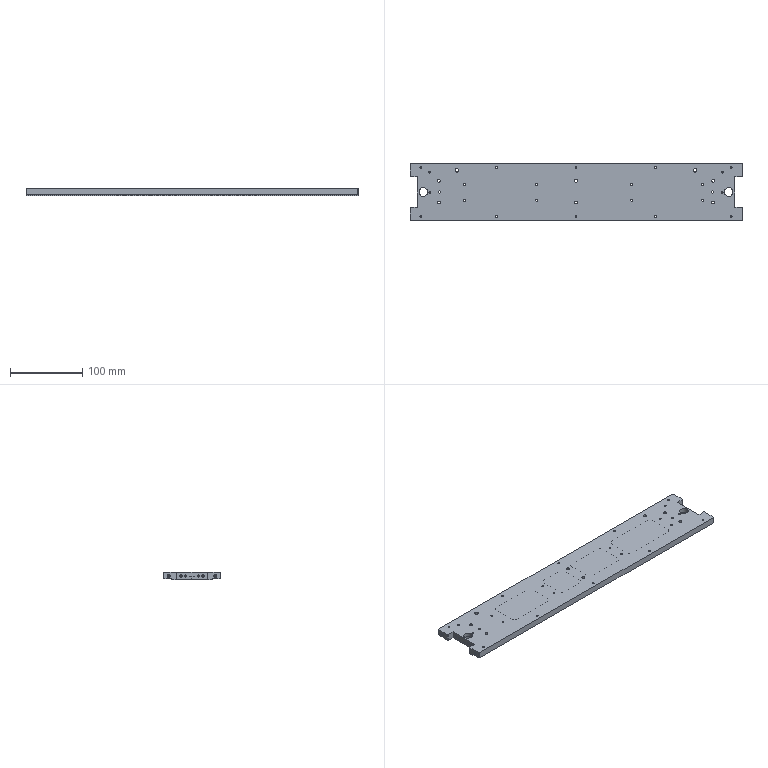Part | NX | features BREP 1 | 1 solid | 179 faces | box 460 x 80 x 10 mm | volume 253015 mm3 | cylinder 107 | plane 52 | cone 20 | commonest cylinder face diameters 2.5 x44 10 x16 3 x12 4 x12 3.3 x8 4.2 x4